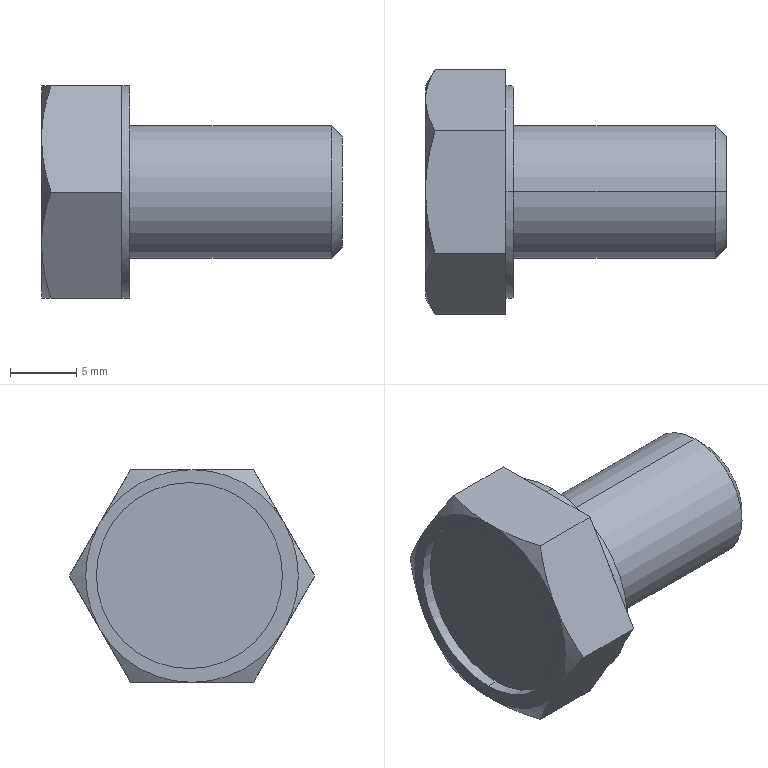Part | STEP file | formed hex screw_am_B18.2.3.2M - Formed hex screw, M10 x 1.5 x 16 --16WN | 1 solid | 30 faces | box 22.63 x 18.475 x 16 mm | volume 2572 mm3 | plane 16 | cone 8 | cylinder 6 | commonest cylinder face diameters 10 x2 14 x2 16 x2